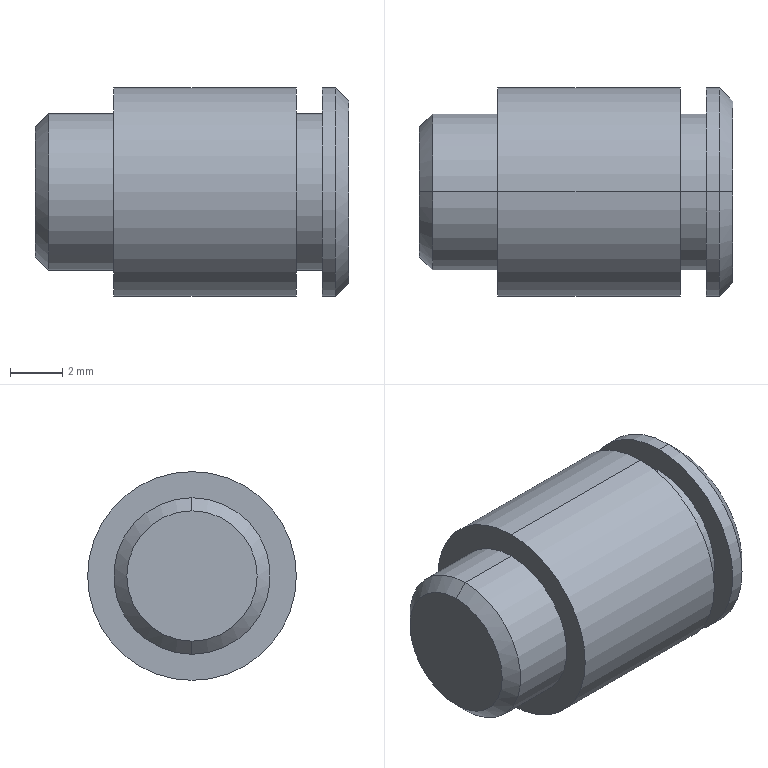Part | STEP file | 1 solid | 17 faces | box 12 x 8 x 8 mm | volume 509.985 mm3 | cylinder 8 | plane 5 | cone 4 | commonest cylinder face diameters 6 x4 8 x4
STEP:
#1=CARTESIAN_POINT('',(0.,0.,0.));
#2=DIRECTION('',(0.,0.,1.));
#3=DIRECTION('',(1.,0.,0.));
#4=AXIS2_PLACEMENT_3D('',#1,#2,#3);
#5=CARTESIAN_POINT('',(3.,0.,-4.));
#6=VERTEX_POINT('',#5);
#7=CARTESIAN_POINT('',(3.,0.,4.));
#8=VERTEX_POINT('',#7);
#9=CARTESIAN_POINT('',(3.,0.,0.));
#10=DIRECTION('',(1.,0.,0.));
#11=DIRECTION('',(0.,0.,-1.));
#12=AXIS2_PLACEMENT_3D('',#9,#10,#11);
#13=CIRCLE('',#12,4.);
#14=CARTESIAN_POINT('',(6.5,0.,0.));
#15=DIRECTION('',(1.,0.,0.));
#16=DIRECTION('',(0.,0.,-1.));
#17=AXIS2_PLACEMENT_3D('',#14,#15,#16);
#18=CYLINDRICAL_SURFACE('',#17,4.);
#19=CARTESIAN_POINT('',(0.,-3.5));
#20=DIRECTION('',(1.,0.));
#21=VECTOR('',#20,1.);
#22=LINE('',#19,#21);
#23=(GEOMETRIC_REPRESENTATION_CONTEXT(2)PARAMETRIC_REPRESENTATION_CONTEXT()REPRESENTATION_CONTEXT('',''));
#24=DEFINITIONAL_REPRESENTATION('',(#22),#23);
#25=PCURVE('',#18,#24);
#26=CARTESIAN_POINT('',(3.,3.5,0.));
#27=DIRECTION('',(-1.,0.,0.));
#28=DIRECTION('',(0.,0.,1.));
#29=AXIS2_PLACEMENT_3D('',#26,#27,#28);
#30=PLANE('',#29);
#31=CARTESIAN_POINT('',(-4.,-3.5));
#32=CARTESIAN_POINT('',(-4.,3.428));
#33=CARTESIAN_POINT('',(2.,-0.0359));
#34=CARTESIAN_POINT('',(8.,-3.5));
#35=CARTESIAN_POINT('',(2.,-6.964));
#36=CARTESIAN_POINT('',(-4.,-10.428));
#37=CARTESIAN_POINT('',(-4.,-3.5));
#38=(BOUNDED_CURVE()B_SPLINE_CURVE(2,(#31,#32,#33,#34,#35,#36,#37),.UNSPECIFIED.,.T.,.F.)B_SPLINE_CURVE_WITH_KNOTS((1,2,2,2,2,1),(-2.094,0.,2.094,4.189,6.283,8.378),.UNSPECIFIED.)CURVE()GEOMETRIC_REPRESENTATION_ITEM()RATIONAL_B_SPLINE_CURVE((1.,0.5,1.,0.5,1.,0.5,1.))REPRESENTATION_ITEM(''));
#39=(GEOMETRIC_REPRESENTATION_CONTEXT(2)PARAMETRIC_REPRESENTATION_CONTEXT()REPRESENTATION_CONTEXT('',''));
#40=DEFINITIONAL_REPRESENTATION('',(#38),#39);
#41=PCURVE('',#30,#40);
#42=SURFACE_CURVE('',#13,(#25,#41),.PCURVE_S1.);
#43=EDGE_CURVE('',#6,#8,#42,.T.);
#44=ORIENTED_EDGE('',*,*,#43,.T.);
#45=CARTESIAN_POINT('',(10.,0.,4.));
#46=VERTEX_POINT('',#45);
#47=CARTESIAN_POINT('',(6.5,0.,4.));
#48=DIRECTION('',(1.,0.,0.));
#49=VECTOR('',#48,1.);
#50=LINE('',#47,#49);
#51=CARTESIAN_POINT('',(3.142,0.));
#52=DIRECTION('',(0.,1.));
#53=VECTOR('',#52,1.);
#54=LINE('',#51,#53);
#55=(GEOMETRIC_REPRESENTATION_CONTEXT(2)PARAMETRIC_REPRESENTATION_CONTEXT()REPRESENTATION_CONTEXT('',''));
#56=DEFINITIONAL_REPRESENTATION('',(#54),#55);
#57=PCURVE('',#18,#56);
#58=CARTESIAN_POINT('',(6.5,0.,0.));
#59=DIRECTION('',(1.,0.,0.));
#60=DIRECTION('',(0.,0.,-1.));
#61=AXIS2_PLACEMENT_3D('',#58,#59,#60);
#62=CYLINDRICAL_SURFACE('',#61,4.);
#63=CARTESIAN_POINT('',(3.142,0.));
#64=DIRECTION('',(0.,1.));
#65=VECTOR('',#64,1.);
#66=LINE('',#63,#65);
#67=(GEOMETRIC_REPRESENTATION_CONTEXT(2)PARAMETRIC_REPRESENTATION_CONTEXT()REPRESENTATION_CONTEXT('',''));
#68=DEFINITIONAL_REPRESENTATION('',(#66),#67);
#69=PCURVE('',#62,#68);
#70=SURFACE_CURVE('',#50,(#57,#69),.PCURVE_S1.);
#71=EDGE_CURVE('',#8,#46,#70,.T.);
#72=ORIENTED_EDGE('',*,*,#71,.T.);
#73=CARTESIAN_POINT('',(10.,0.,-4.));
#74=VERTEX_POINT('',#73);
#75=CARTESIAN_POINT('',(10.,0.,0.));
#76=DIRECTION('',(-1.,0.,0.));
#77=DIRECTION('',(0.,0.,-1.));
#78=AXIS2_PLACEMENT_3D('',#75,#76,#77);
#79=CIRCLE('',#78,4.);
#80=CARTESIAN_POINT('',(6.283,3.5));
#81=DIRECTION('',(-1.,0.));
#82=VECTOR('',#81,1.);
#83=LINE('',#80,#82);
#84=(GEOMETRIC_REPRESENTATION_CONTEXT(2)PARAMETRIC_REPRESENTATION_CONTEXT()REPRESENTATION_CONTEXT('',''));
#85=DEFINITIONAL_REPRESENTATION('',(#83),#84);
#86=PCURVE('',#18,#85);
#87=CARTESIAN_POINT('',(10.,3.5,0.));
#88=DIRECTION('',(1.,0.,0.));
#89=DIRECTION('',(0.,0.,-1.));
#90=AXIS2_PLACEMENT_3D('',#87,#88,#89);
#91=PLANE('',#90);
#92=CARTESIAN_POINT('',(4.,-3.5));
#93=CARTESIAN_POINT('',(4.,-10.428));
#94=CARTESIAN_POINT('',(-2.,-6.964));
#95=CARTESIAN_POINT('',(-8.,-3.5));
#96=CARTESIAN_POINT('',(-2.,-0.0359));
#97=CARTESIAN_POINT('',(4.,3.428));
#98=CARTESIAN_POINT('',(4.,-3.5));
#99=(BOUNDED_CURVE()B_SPLINE_CURVE(2,(#92,#93,#94,#95,#96,#97,#98),.UNSPECIFIED.,.T.,.F.)B_SPLINE_CURVE_WITH_KNOTS((1,2,2,2,2,1),(-2.094,0.,2.094,4.189,6.283,8.378),.UNSPECIFIED.)CURVE()GEOMETRIC_REPRESENTATION_ITEM()RATIONAL_B_SPLINE_CURVE((1.,0.5,1.,0.5,1.,0.5,1.))REPRESENTATION_ITEM(''));
#100=(GEOMETRIC_REPRESENTATION_CONTEXT(2)PARAMETRIC_REPRESENTATION_CONTEXT()REPRESENTATION_CONTEXT('',''));
#101=DEFINITIONAL_REPRESENTATION('',(#99),#100);
#102=PCURVE('',#91,#101);
#103=SURFACE_CURVE('',#79,(#86,#102),.PCURVE_S1.);
#104=EDGE_CURVE('',#46,#74,#103,.T.);
#105=ORIENTED_EDGE('',*,*,#104,.T.);
#106=CARTESIAN_POINT('',(6.5,0.,-4.));
#107=DIRECTION('',(1.,0.,0.));
#108=VECTOR('',#107,1.);
#109=LINE('',#106,#108);
#110=CARTESIAN_POINT('',(0.,0.));
#111=DIRECTION('',(0.,1.));
#112=VECTOR('',#111,1.);
#113=LINE('',#110,#112);
#114=(GEOMETRIC_REPRESENTATION_CONTEXT(2)PARAMETRIC_REPRESENTATION_CONTEXT()REPRESENTATION_CONTEXT('',''));
#115=DEFINITIONAL_REPRESENTATION('',(#113),#114);
#116=PCURVE('',#18,#115);
#117=CARTESIAN_POINT('',(6.283,0.));
#118=DIRECTION('',(0.,1.));
#119=VECTOR('',#118,1.);
#120=LINE('',#117,#119);
#121=(GEOMETRIC_REPRESENTATION_CONTEXT(2)PARAMETRIC_REPRESENTATION_CONTEXT()REPRESENTATION_CONTEXT('',''));
#122=DEFINITIONAL_REPRESENTATION('',(#120),#121);
#123=PCURVE('',#62,#122);
#124=SURFACE_CURVE('',#109,(#116,#123),.PCURVE_S1.);
#125=EDGE_CURVE('',#6,#74,#124,.T.);
#126=ORIENTED_EDGE('',*,*,#125,.F.);
#127=EDGE_LOOP('',(#44,#72,#105,#126));
#128=FACE_BOUND('',#127,.T.);
#129=ADVANCED_FACE('',(#128),#18,.T.);
#130=CARTESIAN_POINT('',(0.5,0.,-3.));
#131=VERTEX_POINT('',#130);
#132=CARTESIAN_POINT('',(0.5,0.,3.));
#133=VERTEX_POINT('',#132);
#134=CARTESIAN_POINT('',(0.5,0.,0.));
#135=DIRECTION('',(1.,0.,0.));
#136=DIRECTION('',(0.,0.,-1.));
#137=AXIS2_PLACEMENT_3D('',#134,#135,#136);
#138=CIRCLE('',#137,3.);
#139=CARTESIAN_POINT('',(1.5,0.,0.));
#140=DIRECTION('',(1.,0.,0.));
#141=DIRECTION('',(0.,0.,-1.));
#142=AXIS2_PLACEMENT_3D('',#139,#140,#141);
#143=CYLINDRICAL_SURFACE('',#142,3.);
#144=CARTESIAN_POINT('',(0.,-1.));
#145=DIRECTION('',(1.,0.));
#146=VECTOR('',#145,1.);
#147=LINE('',#144,#146);
#148=(GEOMETRIC_REPRESENTATION_CONTEXT(2)PARAMETRIC_REPRESENTATION_CONTEXT()REPRESENTATION_CONTEXT('',''));
#149=DEFINITIONAL_REPRESENTATION('',(#147),#148);
#150=PCURVE('',#143,#149);
#151=CARTESIAN_POINT('',(0.5,0.,0.));
#152=DIRECTION('',(1.,0.,0.));
#153=DIRECTION('',(0.,0.,-1.));
#154=AXIS2_PLACEMENT_3D('',#151,#152,#153);
#155=CONICAL_SURFACE('',#154,3.,0.7854);
#156=CARTESIAN_POINT('',(0.,0.));
#157=DIRECTION('',(1.,0.));
#158=VECTOR('',#157,1.);
#159=LINE('',#156,#158);
#160=(GEOMETRIC_REPRESENTATION_CONTEXT(2)PARAMETRIC_REPRESENTATION_CONTEXT()REPRESENTATION_CONTEXT('',''));
#161=DEFINITIONAL_REPRESENTATION('',(#159),#160);
#162=PCURVE('',#155,#161);
#163=SURFACE_CURVE('',#138,(#150,#162),.PCURVE_S1.);
#164=EDGE_CURVE('',#131,#133,#163,.T.);
#165=ORIENTED_EDGE('',*,*,#164,.T.);
#166=CARTESIAN_POINT('',(3.,0.,3.));
#167=VERTEX_POINT('',#166);
#168=CARTESIAN_POINT('',(1.5,0.,3.));
#169=DIRECTION('',(1.,0.,0.));
#170=VECTOR('',#169,1.);
#171=LINE('',#168,#170);
#172=CARTESIAN_POINT('',(3.142,0.));
#173=DIRECTION('',(0.,1.));
#174=VECTOR('',#173,1.);
#175=LINE('',#172,#174);
#176=(GEOMETRIC_REPRESENTATION_CONTEXT(2)PARAMETRIC_REPRESENTATION_CONTEXT()REPRESENTATION_CONTEXT('',''));
#177=DEFINITIONAL_REPRESENTATION('',(#175),#176);
#178=PCURVE('',#143,#177);
#179=CARTESIAN_POINT('',(1.5,0.,0.));
#180=DIRECTION('',(1.,0.,0.));
#181=DIRECTION('',(0.,0.,-1.));
#182=AXIS2_PLACEMENT_3D('',#179,#180,#181);
#183=CYLINDRICAL_SURFACE('',#182,3.);
#184=CARTESIAN_POINT('',(3.142,0.));
#185=DIRECTION('',(0.,1.));
#186=VECTOR('',#185,1.);
#187=LINE('',#184,#186);
#188=(GEOMETRIC_REPRESENTATION_CONTEXT(2)PARAMETRIC_REPRESENTATION_CONTEXT()REPRESENTATION_CONTEXT('',''));
#189=DEFINITIONAL_REPRESENTATION('',(#187),#188);
#190=PCURVE('',#183,#189);
#191=SURFACE_CURVE('',#171,(#178,#190),.PCURVE_S1.);
#192=EDGE_CURVE('',#133,#167,#191,.T.);
#193=ORIENTED_EDGE('',*,*,#192,.T.);
#194=CARTESIAN_POINT('',(3.,0.,-3.));
#195=VERTEX_POINT('',#194);
#196=CARTESIAN_POINT('',(3.,0.,0.));
#197=DIRECTION('',(1.,0.,0.));
#198=DIRECTION('',(0.,0.,-1.));
#199=AXIS2_PLACEMENT_3D('',#196,#197,#198);
#200=CIRCLE('',#199,3.);
#201=CARTESIAN_POINT('',(0.,1.5));
#202=DIRECTION('',(1.,0.));
#203=VECTOR('',#202,1.);
#204=LINE('',#201,#203);
#205=(GEOMETRIC_REPRESENTATION_CONTEXT(2)PARAMETRIC_REPRESENTATION_CONTEXT()REPRESENTATION_CONTEXT('',''));
#206=DEFINITIONAL_REPRESENTATION('',(#204),#205);
#207=PCURVE('',#143,#206);
#208=CARTESIAN_POINT('',(-3.,-3.5));
#209=CARTESIAN_POINT('',(-3.,1.696));
#210=CARTESIAN_POINT('',(1.5,-0.9019));
#211=CARTESIAN_POINT('',(6.,-3.5));
#212=CARTESIAN_POINT('',(1.5,-6.098));
#213=CARTESIAN_POINT('',(-3.,-8.696));
#214=CARTESIAN_POINT('',(-3.,-3.5));
#215=(BOUNDED_CURVE()B_SPLINE_CURVE(2,(#208,#209,#210,#211,#212,#213,#214),.UNSPECIFIED.,.T.,.F.)B_SPLINE_CURVE_WITH_KNOTS((1,2,2,2,2,1),(-2.094,0.,2.094,4.189,6.283,8.378),.UNSPECIFIED.)CURVE()GEOMETRIC_REPRESENTATION_ITEM()RATIONAL_B_SPLINE_CURVE((1.,0.5,1.,0.5,1.,0.5,1.))REPRESENTATION_ITEM(''));
#216=(GEOMETRIC_REPRESENTATION_CONTEXT(2)PARAMETRIC_REPRESENTATION_CONTEXT()REPRESENTATION_CONTEXT('',''));
#217=DEFINITIONAL_REPRESENTATION('',(#215),#216);
#218=PCURVE('',#30,#217);
#219=SURFACE_CURVE('',#200,(#207,#218),.PCURVE_S1.);
#220=EDGE_CURVE('',#195,#167,#219,.T.);
#221=ORIENTED_EDGE('',*,*,#220,.F.);
#222=CARTESIAN_POINT('',(1.5,0.,-3.));
#223=DIRECTION('',(1.,0.,0.));
#224=VECTOR('',#223,1.);
#225=LINE('',#222,#224);
#226=CARTESIAN_POINT('',(0.,0.));
#227=DIRECTION('',(0.,1.));
#228=VECTOR('',#227,1.);
#229=LINE('',#226,#228);
#230=(GEOMETRIC_REPRESENTATION_CONTEXT(2)PARAMETRIC_REPRESENTATION_CONTEXT()REPRESENTATION_CONTEXT('',''));
#231=DEFINITIONAL_REPRESENTATION('',(#229),#230);
#232=PCURVE('',#143,#231);
#233=CARTESIAN_POINT('',(6.283,0.));
#234=DIRECTION('',(0.,1.));
#235=VECTOR('',#234,1.);
#236=LINE('',#233,#235);
#237=(GEOMETRIC_REPRESENTATION_CONTEXT(2)PARAMETRIC_REPRESENTATION_CONTEXT()REPRESENTATION_CONTEXT('',''));
#238=DEFINITIONAL_REPRESENTATION('',(#236),#237);
#239=PCURVE('',#183,#238);
#240=SURFACE_CURVE('',#225,(#232,#239),.PCURVE_S1.);
#241=EDGE_CURVE('',#131,#195,#240,.T.);
#242=ORIENTED_EDGE('',*,*,#241,.F.);
#243=EDGE_LOOP('',(#165,#193,#221,#242));
#244=FACE_BOUND('',#243,.T.);
#245=ADVANCED_FACE('',(#244),#143,.T.);
#246=CARTESIAN_POINT('',(10.,0.,3.));
#247=VERTEX_POINT('',#246);
#248=CARTESIAN_POINT('',(10.,0.,-3.));
#249=VERTEX_POINT('',#248);
#250=CARTESIAN_POINT('',(10.,0.,0.));
#251=DIRECTION('',(-1.,0.,0.));
#252=DIRECTION('',(0.,0.,-1.));
#253=AXIS2_PLACEMENT_3D('',#250,#251,#252);
#254=CIRCLE('',#253,3.);
#255=CARTESIAN_POINT('',(10.5,0.,0.));
#256=DIRECTION('',(1.,0.,0.));
#257=DIRECTION('',(0.,0.,-1.));
#258=AXIS2_PLACEMENT_3D('',#255,#256,#257);
#259=CYLINDRICAL_SURFACE('',#258,3.);
#260=CARTESIAN_POINT('',(6.283,-0.5));
#261=DIRECTION('',(-1.,0.));
#262=VECTOR('',#261,1.);
#263=LINE('',#260,#262);
#264=(GEOMETRIC_REPRESENTATION_CONTEXT(2)PARAMETRIC_REPRESENTATION_CONTEXT()REPRESENTATION_CONTEXT('',''));
#265=DEFINITIONAL_REPRESENTATION('',(#263),#264);
#266=PCURVE('',#259,#265);
#267=CARTESIAN_POINT('',(3.,-3.5));
#268=CARTESIAN_POINT('',(3.,-8.696));
#269=CARTESIAN_POINT('',(-1.5,-6.098));
#270=CARTESIAN_POINT('',(-6.,-3.5));
#271=CARTESIAN_POINT('',(-1.5,-0.9019));
#272=CARTESIAN_POINT('',(3.,1.696));
#273=CARTESIAN_POINT('',(3.,-3.5));
#274=(BOUNDED_CURVE()B_SPLINE_CURVE(2,(#267,#268,#269,#270,#271,#272,#273),.UNSPECIFIED.,.T.,.F.)B_SPLINE_CURVE_WITH_KNOTS((1,2,2,2,2,1),(-2.094,0.,2.094,4.189,6.283,8.378),.UNSPECIFIED.)CURVE()GEOMETRIC_REPRESENTATION_ITEM()RATIONAL_B_SPLINE_CURVE((1.,0.5,1.,0.5,1.,0.5,1.))REPRESENTATION_ITEM(''));
#275=(GEOMETRIC_REPRESENTATION_CONTEXT(2)PARAMETRIC_REPRESENTATION_CONTEXT()REPRESENTATION_CONTEXT('',''));
#276=DEFINITIONAL_REPRESENTATION('',(#274),#275);
#277=PCURVE('',#91,#276);
#278=SURFACE_CURVE('',#254,(#266,#277),.PCURVE_S1.);
#279=EDGE_CURVE('',#247,#249,#278,.T.);
#280=ORIENTED_EDGE('',*,*,#279,.F.);
#281=CARTESIAN_POINT('',(11.,0.,3.));
#282=VERTEX_POINT('',#281);
#283=CARTESIAN_POINT('',(10.5,0.,3.));
#284=DIRECTION('',(1.,0.,0.));
#285=VECTOR('',#284,1.);
#286=LINE('',#283,#285);
#287=CARTESIAN_POINT('',(3.142,0.));
#288=DIRECTION('',(0.,1.));
#289=VECTOR('',#288,1.);
#290=LINE('',#287,#289);
#291=(GEOMETRIC_REPRESENTATION_CONTEXT(2)PARAMETRIC_REPRESENTATION_CONTEXT()REPRESENTATION_CONTEXT('',''));
#292=DEFINITIONAL_REPRESENTATION('',(#290),#291);
#293=PCURVE('',#259,#292);
#294=CARTESIAN_POINT('',(10.5,0.,0.));
#295=DIRECTION('',(1.,0.,0.));
#296=DIRECTION('',(0.,0.,-1.));
#297=AXIS2_PLACEMENT_3D('',#294,#295,#296);
#298=CYLINDRICAL_SURFACE('',#297,3.);
#299=CARTESIAN_POINT('',(3.142,0.));
#300=DIRECTION('',(0.,1.));
#301=VECTOR('',#300,1.);
#302=LINE('',#299,#301);
#303=(GEOMETRIC_REPRESENTATION_CONTEXT(2)PARAMETRIC_REPRESENTATION_CONTEXT()REPRESENTATION_CONTEXT('',''));
#304=DEFINITIONAL_REPRESENTATION('',(#302),#303);
#305=PCURVE('',#298,#304);
#306=SURFACE_CURVE('',#286,(#293,#305),.PCURVE_S1.);
#307=EDGE_CURVE('',#247,#282,#306,.T.);
#308=ORIENTED_EDGE('',*,*,#307,.T.);
#309=CARTESIAN_POINT('',(11.,0.,-3.));
#310=VERTEX_POINT('',#309);
#311=CARTESIAN_POINT('',(11.,0.,0.));
#312=DIRECTION('',(-1.,0.,0.));
#313=DIRECTION('',(0.,0.,-1.));
#314=AXIS2_PLACEMENT_3D('',#311,#312,#313);
#315=CIRCLE('',#314,3.);
#316=CARTESIAN_POINT('',(6.283,0.5));
#317=DIRECTION('',(-1.,0.));
#318=VECTOR('',#317,1.);
#319=LINE('',#316,#318);
#320=(GEOMETRIC_REPRESENTATION_CONTEXT(2)PARAMETRIC_REPRESENTATION_CONTEXT()REPRESENTATION_CONTEXT('',''));
#321=DEFINITIONAL_REPRESENTATION('',(#319),#320);
#322=PCURVE('',#259,#321);
#323=CARTESIAN_POINT('',(11.,3.5,0.));
#324=DIRECTION('',(-1.,0.,0.));
#325=DIRECTION('',(0.,0.,1.));
#326=AXIS2_PLACEMENT_3D('',#323,#324,#325);
#327=PLANE('',#326);
#328=CARTESIAN_POINT('',(0.,-3.5));
#329=DIRECTION('',(-1.,0.));
#330=AXIS2_PLACEMENT_2D('',#328,#329);
#331=CIRCLE('',#330,3.);
#332=(GEOMETRIC_REPRESENTATION_CONTEXT(2)PARAMETRIC_REPRESENTATION_CONTEXT()REPRESENTATION_CONTEXT('',''));
#333=DEFINITIONAL_REPRESENTATION('',(#331),#332);
#334=PCURVE('',#327,#333);
#335=SURFACE_CURVE('',#315,(#322,#334),.PCURVE_S1.);
#336=EDGE_CURVE('',#282,#310,#335,.T.);
#337=ORIENTED_EDGE('',*,*,#336,.T.);
#338=CARTESIAN_POINT('',(10.5,0.,-3.));
#339=DIRECTION('',(1.,0.,0.));
#340=VECTOR('',#339,1.);
#341=LINE('',#338,#340);
#342=CARTESIAN_POINT('',(0.,0.));
#343=DIRECTION('',(0.,1.));
#344=VECTOR('',#343,1.);
#345=LINE('',#342,#344);
#346=(GEOMETRIC_REPRESENTATION_CONTEXT(2)PARAMETRIC_REPRESENTATION_CONTEXT()REPRESENTATION_CONTEXT('',''));
#347=DEFINITIONAL_REPRESENTATION('',(#345),#346);
#348=PCURVE('',#259,#347);
#349=CARTESIAN_POINT('',(6.283,0.));
#350=DIRECTION('',(0.,1.));
#351=VECTOR('',#350,1.);
#352=LINE('',#349,#351);
#353=(GEOMETRIC_REPRESENTATION_CONTEXT(2)PARAMETRIC_REPRESENTATION_CONTEXT()REPRESENTATION_CONTEXT('',''));
#354=DEFINITIONAL_REPRESENTATION('',(#352),#353);
#355=PCURVE('',#298,#354);
#356=SURFACE_CURVE('',#341,(#348,#355),.PCURVE_S1.);
#357=EDGE_CURVE('',#249,#310,#356,.T.);
#358=ORIENTED_EDGE('',*,*,#357,.F.);
#359=EDGE_LOOP('',(#280,#308,#337,#358));
#360=FACE_BOUND('',#359,.T.);
#361=ADVANCED_FACE('',(#360),#259,.T.);
#362=CARTESIAN_POINT('',(0.,0.,-2.5));
#363=VERTEX_POINT('',#362);
#364=CARTESIAN_POINT('',(0.,0.,2.5));
#365=VERTEX_POINT('',#364);
#366=CARTESIAN_POINT('',(0.,0.,0.));
#367=DIRECTION('',(1.,0.,0.));
#368=DIRECTION('',(0.,0.,-1.));
#369=AXIS2_PLACEMENT_3D('',#366,#367,#368);
#370=CIRCLE('',#369,2.5);
#371=CARTESIAN_POINT('',(0.,-0.5));
#372=DIRECTION('',(1.,0.));
#373=VECTOR('',#372,1.);
#374=LINE('',#371,#373);
#375=(GEOMETRIC_REPRESENTATION_CONTEXT(2)PARAMETRIC_REPRESENTATION_CONTEXT()REPRESENTATION_CONTEXT('',''));
#376=DEFINITIONAL_REPRESENTATION('',(#374),#375);
#377=PCURVE('',#155,#376);
#378=CARTESIAN_POINT('',(0.,1.5,0.));
#379=DIRECTION('',(-1.,0.,0.));
#380=DIRECTION('',(0.,0.,1.));
#381=AXIS2_PLACEMENT_3D('',#378,#379,#380);
#382=PLANE('',#381);
#383=CARTESIAN_POINT('',(-2.5,-1.5));
#384=CARTESIAN_POINT('',(-2.5,2.83));
#385=CARTESIAN_POINT('',(1.25,0.6651));
#386=CARTESIAN_POINT('',(5.,-1.5));
#387=CARTESIAN_POINT('',(1.25,-3.665));
#388=CARTESIAN_POINT('',(-2.5,-5.83));
#389=CARTESIAN_POINT('',(-2.5,-1.5));
#390=(BOUNDED_CURVE()B_SPLINE_CURVE(2,(#383,#384,#385,#386,#387,#388,#389),.UNSPECIFIED.,.T.,.F.)B_SPLINE_CURVE_WITH_KNOTS((1,2,2,2,2,1),(-2.094,0.,2.094,4.189,6.283,8.378),.UNSPECIFIED.)CURVE()GEOMETRIC_REPRESENTATION_ITEM()RATIONAL_B_SPLINE_CURVE((1.,0.5,1.,0.5,1.,0.5,1.))REPRESENTATION_ITEM(''));
#391=(GEOMETRIC_REPRESENTATION_CONTEXT(2)PARAMETRIC_REPRESENTATION_CONTEXT()REPRESENTATION_CONTEXT('',''));
#392=DEFINITIONAL_REPRESENTATION('',(#390),#391);
#393=PCURVE('',#382,#392);
#394=SURFACE_CURVE('',#370,(#377,#393),.PCURVE_S1.);
#395=EDGE_CURVE('',#363,#365,#394,.T.);
#396=ORIENTED_EDGE('',*,*,#395,.T.);
#397=CARTESIAN_POINT('',(0.5,0.,3.));
#398=DIRECTION('',(0.7071,0.,0.7071));
#399=VECTOR('',#398,1.);
#400=LINE('',#397,#399);
#401=CARTESIAN_POINT('',(3.142,0.));
#402=DIRECTION('',(0.,1.));
#403=VECTOR('',#402,1.);
#404=LINE('',#401,#403);
#405=(GEOMETRIC_REPRESENTATION_CONTEXT(2)PARAMETRIC_REPRESENTATION_CONTEXT()REPRESENTATION_CONTEXT('',''));
#406=DEFINITIONAL_REPRESENTATION('',(#404),#405);
#407=PCURVE('',#155,#406);
#408=CARTESIAN_POINT('',(0.5,0.,0.));
#409=DIRECTION('',(1.,0.,0.));
#410=DIRECTION('',(0.,0.,-1.));
#411=AXIS2_PLACEMENT_3D('',#408,#409,#410);
#412=CONICAL_SURFACE('',#411,3.,0.7854);
#413=CARTESIAN_POINT('',(3.142,0.));
#414=DIRECTION('',(0.,1.));
#415=VECTOR('',#414,1.);
#416=LINE('',#413,#415);
#417=(GEOMETRIC_REPRESENTATION_CONTEXT(2)PARAMETRIC_REPRESENTATION_CONTEXT()REPRESENTATION_CONTEXT('',''));
#418=DEFINITIONAL_REPRESENTATION('',(#416),#417);
#419=PCURVE('',#412,#418);
#420=SURFACE_CURVE('',#400,(#407,#419),.PCURVE_S1.);
#421=EDGE_CURVE('',#365,#133,#420,.T.);
#422=ORIENTED_EDGE('',*,*,#421,.T.);
#423=ORIENTED_EDGE('',*,*,#164,.F.);
#424=CARTESIAN_POINT('',(0.5,0.,-3.));
#425=DIRECTION('',(0.7071,0.,-0.7071));
#426=VECTOR('',#425,1.);
#427=LINE('',#424,#426);
#428=CARTESIAN_POINT('',(0.,0.));
#429=DIRECTION('',(0.,1.));
#430=VECTOR('',#429,1.);
#431=LINE('',#428,#430);
#432=(GEOMETRIC_REPRESENTATION_CONTEXT(2)PARAMETRIC_REPRESENTATION_CONTEXT()REPRESENTATION_CONTEXT('',''));
#433=DEFINITIONAL_REPRESENTATION('',(#431),#432);
#434=PCURVE('',#155,#433);
#435=CARTESIAN_POINT('',(6.283,0.));
#436=DIRECTION('',(0.,1.));
#437=VECTOR('',#436,1.);
#438=LINE('',#435,#437);
#439=(GEOMETRIC_REPRESENTATION_CONTEXT(2)PARAMETRIC_REPRESENTATION_CONTEXT()REPRESENTATION_CONTEXT('',''));
#440=DEFINITIONAL_REPRESENTATION('',(#438),#439);
#441=PCURVE('',#412,#440);
#442=SURFACE_CURVE('',#427,(#434,#441),.PCURVE_S1.);
#443=EDGE_CURVE('',#363,#131,#442,.T.);
#444=ORIENTED_EDGE('',*,*,#443,.F.);
#445=EDGE_LOOP('',(#396,#422,#423,#444));
#446=FACE_BOUND('',#445,.T.);
#447=ADVANCED_FACE('',(#446),#155,.T.);
#448=CARTESIAN_POINT('',(11.,0.,4.));
#449=VERTEX_POINT('',#448);
#450=CARTESIAN_POINT('',(11.,0.,-4.));
#451=VERTEX_POINT('',#450);
#452=CARTESIAN_POINT('',(11.,0.,0.));
#453=DIRECTION('',(-1.,0.,0.));
#454=DIRECTION('',(0.,0.,-1.));
#455=AXIS2_PLACEMENT_3D('',#452,#453,#454);
#456=CIRCLE('',#455,4.);
#457=CARTESIAN_POINT('',(11.5,0.,0.));
#458=DIRECTION('',(1.,0.,0.));
#459=DIRECTION('',(0.,0.,-1.));
#460=AXIS2_PLACEMENT_3D('',#457,#458,#459);
#461=CYLINDRICAL_SURFACE('',#460,4.);
#462=CARTESIAN_POINT('',(6.283,-0.5));
#463=DIRECTION('',(-1.,0.));
#464=VECTOR('',#463,1.);
#465=LINE('',#462,#464);
#466=(GEOMETRIC_REPRESENTATION_CONTEXT(2)PARAMETRIC_REPRESENTATION_CONTEXT()REPRESENTATION_CONTEXT('',''));
#467=DEFINITIONAL_REPRESENTATION('',(#465),#466);
#468=PCURVE('',#461,#467);
#469=CARTESIAN_POINT('',(0.,-3.5));
#470=DIRECTION('',(-1.,0.));
#471=AXIS2_PLACEMENT_2D('',#469,#470);
#472=CIRCLE('',#471,4.);
#473=(GEOMETRIC_REPRESENTATION_CONTEXT(2)PARAMETRIC_REPRESENTATION_CONTEXT()REPRESENTATION_CONTEXT('',''));
#474=DEFINITIONAL_REPRESENTATION('',(#472),#473);
#475=PCURVE('',#327,#474);
#476=SURFACE_CURVE('',#456,(#468,#475),.PCURVE_S1.);
#477=EDGE_CURVE('',#449,#451,#476,.T.);
#478=ORIENTED_EDGE('',*,*,#477,.F.);
#479=CARTESIAN_POINT('',(11.5,0.,4.));
#480=VERTEX_POINT('',#479);
#481=CARTESIAN_POINT('',(11.5,0.,4.));
#482=DIRECTION('',(1.,0.,0.));
#483=VECTOR('',#482,1.);
#484=LINE('',#481,#483);
#485=CARTESIAN_POINT('',(3.142,0.));
#486=DIRECTION('',(0.,1.));
#487=VECTOR('',#486,1.);
#488=LINE('',#485,#487);
#489=(GEOMETRIC_REPRESENTATION_CONTEXT(2)PARAMETRIC_REPRESENTATION_CONTEXT()REPRESENTATION_CONTEXT('',''));
#490=DEFINITIONAL_REPRESENTATION('',(#488),#489);
#491=PCURVE('',#461,#490);
#492=CARTESIAN_POINT('',(11.5,0.,0.));
#493=DIRECTION('',(1.,0.,0.));
#494=DIRECTION('',(0.,0.,-1.));
#495=AXIS2_PLACEMENT_3D('',#492,#493,#494);
#496=CYLINDRICAL_SURFACE('',#495,4.);
#497=CARTESIAN_POINT('',(3.142,0.));
#498=DIRECTION('',(0.,1.));
#499=VECTOR('',#498,1.);
#500=LINE('',#497,#499);
#501=(GEOMETRIC_REPRESENTATION_CONTEXT(2)PARAMETRIC_REPRESENTATION_CONTEXT()REPRESENTATION_CONTEXT('',''));
#502=DEFINITIONAL_REPRESENTATION('',(#500),#501);
#503=PCURVE('',#496,#502);
#504=SURFACE_CURVE('',#484,(#491,#503),.PCURVE_S1.);
#505=EDGE_CURVE('',#449,#480,#504,.T.);
#506=ORIENTED_EDGE('',*,*,#505,.T.);
#507=CARTESIAN_POINT('',(11.5,0.,-4.));
#508=VERTEX_POINT('',#507);
#509=CARTESIAN_POINT('',(11.5,0.,0.));
#510=DIRECTION('',(-1.,0.,0.));
#511=DIRECTION('',(0.,0.,-1.));
#512=AXIS2_PLACEMENT_3D('',#509,#510,#511);
#513=CIRCLE('',#512,4.);
#514=CARTESIAN_POINT('',(6.283,0.));
#515=DIRECTION('',(-1.,0.));
#516=VECTOR('',#515,1.);
#517=LINE('',#514,#516);
#518=(GEOMETRIC_REPRESENTATION_CONTEXT(2)PARAMETRIC_REPRESENTATION_CONTEXT()REPRESENTATION_CONTEXT('',''));
#519=DEFINITIONAL_REPRESENTATION('',(#517),#518);
#520=PCURVE('',#461,#519);
#521=CARTESIAN_POINT('',(11.5,0.,0.));
#522=DIRECTION('',(-1.,0.,0.));
#523=DIRECTION('',(0.,0.,1.));
#524=AXIS2_PLACEMENT_3D('',#521,#522,#523);
#525=CONICAL_SURFACE('',#524,4.,0.7854);
#526=CARTESIAN_POINT('',(-3.142,0.));
#527=DIRECTION('',(1.,0.));
#528=VECTOR('',#527,1.);
#529=LINE('',#526,#528);
#530=(GEOMETRIC_REPRESENTATION_CONTEXT(2)PARAMETRIC_REPRESENTATION_CONTEXT()REPRESENTATION_CONTEXT('',''));
#531=DEFINITIONAL_REPRESENTATION('',(#529),#530);
#532=PCURVE('',#525,#531);
#533=SURFACE_CURVE('',#513,(#520,#532),.PCURVE_S1.);
#534=EDGE_CURVE('',#480,#508,#533,.T.);
#535=ORIENTED_EDGE('',*,*,#534,.T.);
#536=CARTESIAN_POINT('',(11.5,0.,-4.));
#537=DIRECTION('',(1.,0.,0.));
#538=VECTOR('',#537,1.);
#539=LINE('',#536,#538);
#540=CARTESIAN_POINT('',(0.,0.));
#541=DIRECTION('',(0.,1.));
#542=VECTOR('',#541,1.);
#543=LINE('',#540,#542);
#544=(GEOMETRIC_REPRESENTATION_CONTEXT(2)PARAMETRIC_REPRESENTATION_CONTEXT()REPRESENTATION_CONTEXT('',''));
#545=DEFINITIONAL_REPRESENTATION('',(#543),#544);
#546=PCURVE('',#461,#545);
#547=CARTESIAN_POINT('',(6.283,0.));
#548=DIRECTION('',(0.,1.));
#549=VECTOR('',#548,1.);
#550=LINE('',#547,#549);
#551=(GEOMETRIC_REPRESENTATION_CONTEXT(2)PARAMETRIC_REPRESENTATION_CONTEXT()REPRESENTATION_CONTEXT('',''));
#552=DEFINITIONAL_REPRESENTATION('',(#550),#551);
#553=PCURVE('',#496,#552);
#554=SURFACE_CURVE('',#539,(#546,#553),.PCURVE_S1.);
#555=EDGE_CURVE('',#451,#508,#554,.T.);
#556=ORIENTED_EDGE('',*,*,#555,.F.);
#557=EDGE_LOOP('',(#478,#506,#535,#556));
#558=FACE_BOUND('',#557,.T.);
#559=ADVANCED_FACE('',(#558),#461,.T.);
#560=CARTESIAN_POINT('',(12.,0.,3.5));
#561=VERTEX_POINT('',#560);
#562=CARTESIAN_POINT('',(12.,0.,-3.5));
#563=VERTEX_POINT('',#562);
#564=CARTESIAN_POINT('',(12.,0.,0.));
#565=DIRECTION('',(-1.,0.,0.));
#566=DIRECTION('',(0.,0.,1.));
#567=AXIS2_PLACEMENT_3D('',#564,#565,#566);
#568=CIRCLE('',#567,3.5);
#569=CARTESIAN_POINT('',(0.,-0.5));
#570=DIRECTION('',(1.,0.));
#571=VECTOR('',#570,1.);
#572=LINE('',#569,#571);
#573=(GEOMETRIC_REPRESENTATION_CONTEXT(2)PARAMETRIC_REPRESENTATION_CONTEXT()REPRESENTATION_CONTEXT('',''));
#574=DEFINITIONAL_REPRESENTATION('',(#572),#573);
#575=PCURVE('',#525,#574);
#576=CARTESIAN_POINT('',(12.,2.,0.));
#577=DIRECTION('',(1.,0.,0.));
#578=DIRECTION('',(0.,0.,-1.));
#579=AXIS2_PLACEMENT_3D('',#576,#577,#578);
#580=PLANE('',#579);
#581=CARTESIAN_POINT('',(-3.5,-2.));
#582=CARTESIAN_POINT('',(-3.5,4.062));
#583=CARTESIAN_POINT('',(1.75,1.031));
#584=CARTESIAN_POINT('',(7.,-2.));
#585=CARTESIAN_POINT('',(1.75,-5.031));
#586=CARTESIAN_POINT('',(-3.5,-8.062));
#587=CARTESIAN_POINT('',(-3.5,-2.));
#588=(BOUNDED_CURVE()B_SPLINE_CURVE(2,(#581,#582,#583,#584,#585,#586,#587),.UNSPECIFIED.,.T.,.F.)B_SPLINE_CURVE_WITH_KNOTS((1,2,2,2,2,1),(-2.094,0.,2.094,4.189,6.283,8.378),.UNSPECIFIED.)CURVE()GEOMETRIC_REPRESENTATION_ITEM()RATIONAL_B_SPLINE_CURVE((1.,0.5,1.,0.5,1.,0.5,1.))REPRESENTATION_ITEM(''));
#589=(GEOMETRIC_REPRESENTATION_CONTEXT(2)PARAMETRIC_REPRESENTATION_CONTEXT()REPRESENTATION_CONTEXT('',''));
#590=DEFINITIONAL_REPRESENTATION('',(#588),#589);
#591=PCURVE('',#580,#590);
#592=SURFACE_CURVE('',#568,(#575,#591),.PCURVE_S1.);
#593=EDGE_CURVE('',#561,#563,#592,.T.);
#594=ORIENTED_EDGE('',*,*,#593,.T.);
#595=CARTESIAN_POINT('',(11.5,0.,-4.));
#596=DIRECTION('',(-0.7071,0.,-0.7071));
#597=VECTOR('',#596,1.);
#598=LINE('',#595,#597);
#599=CARTESIAN_POINT('',(3.142,0.));
#600=DIRECTION('',(0.,1.));
#601=VECTOR('',#600,1.);
#602=LINE('',#599,#601);
#603=(GEOMETRIC_REPRESENTATION_CONTEXT(2)PARAMETRIC_REPRESENTATION_CONTEXT()REPRESENTATION_CONTEXT('',''));
#604=DEFINITIONAL_REPRESENTATION('',(#602),#603);
#605=PCURVE('',#525,#604);
#606=CARTESIAN_POINT('',(11.5,0.,0.));
#607=DIRECTION('',(-1.,0.,0.));
#608=DIRECTION('',(0.,0.,1.));
#609=AXIS2_PLACEMENT_3D('',#606,#607,#608);
#610=CONICAL_SURFACE('',#609,4.,0.7854);
#611=CARTESIAN_POINT('',(3.142,0.));
#612=DIRECTION('',(0.,1.));
#613=VECTOR('',#612,1.);
#614=LINE('',#611,#613);
#615=(GEOMETRIC_REPRESENTATION_CONTEXT(2)PARAMETRIC_REPRESENTATION_CONTEXT()REPRESENTATION_CONTEXT('',''));
#616=DEFINITIONAL_REPRESENTATION('',(#614),#615);
#617=PCURVE('',#610,#616);
#618=SURFACE_CURVE('',#598,(#605,#617),.PCURVE_S1.);
#619=EDGE_CURVE('',#563,#508,#618,.T.);
#620=ORIENTED_EDGE('',*,*,#619,.T.);
#621=ORIENTED_EDGE('',*,*,#534,.F.);
#622=CARTESIAN_POINT('',(11.5,0.,4.));
#623=DIRECTION('',(-0.7071,0.,0.7071));
#624=VECTOR('',#623,1.);
#625=LINE('',#622,#624);
#626=CARTESIAN_POINT('',(0.,0.));
#627=DIRECTION('',(0.,1.));
#628=VECTOR('',#627,1.);
#629=LINE('',#626,#628);
#630=(GEOMETRIC_REPRESENTATION_CONTEXT(2)PARAMETRIC_REPRESENTATION_CONTEXT()REPRESENTATION_CONTEXT('',''));
#631=DEFINITIONAL_REPRESENTATION('',(#629),#630);
#632=PCURVE('',#525,#631);
#633=CARTESIAN_POINT('',(6.283,0.));
#634=DIRECTION('',(0.,1.));
#635=VECTOR('',#634,1.);
#636=LINE('',#633,#635);
#637=(GEOMETRIC_REPRESENTATION_CONTEXT(2)PARAMETRIC_REPRESENTATION_CONTEXT()REPRESENTATION_CONTEXT('',''));
#638=DEFINITIONAL_REPRESENTATION('',(#636),#637);
#639=PCURVE('',#610,#638);
#640=SURFACE_CURVE('',#625,(#632,#639),.PCURVE_S1.);
#641=EDGE_CURVE('',#561,#480,#640,.T.);
#642=ORIENTED_EDGE('',*,*,#641,.F.);
#643=EDGE_LOOP('',(#594,#620,#621,#642));
#644=FACE_BOUND('',#643,.T.);
#645=ADVANCED_FACE('',(#644),#525,.T.);
#646=ORIENTED_EDGE('',*,*,#71,.F.);
#647=CARTESIAN_POINT('',(3.,0.,0.));
#648=DIRECTION('',(1.,0.,0.));
#649=DIRECTION('',(0.,0.,-1.));
#650=AXIS2_PLACEMENT_3D('',#647,#648,#649);
#651=CIRCLE('',#650,4.);
#652=CARTESIAN_POINT('',(0.,-3.5));
#653=DIRECTION('',(1.,0.));
#654=VECTOR('',#653,1.);
#655=LINE('',#652,#654);
#656=(GEOMETRIC_REPRESENTATION_CONTEXT(2)PARAMETRIC_REPRESENTATION_CONTEXT()REPRESENTATION_CONTEXT('',''));
#657=DEFINITIONAL_REPRESENTATION('',(#655),#656);
#658=PCURVE('',#62,#657);
#659=CARTESIAN_POINT('',(-4.,-3.5));
#660=CARTESIAN_POINT('',(-4.,3.428));
#661=CARTESIAN_POINT('',(2.,-0.0359));
#662=CARTESIAN_POINT('',(8.,-3.5));
#663=CARTESIAN_POINT('',(2.,-6.964));
#664=CARTESIAN_POINT('',(-4.,-10.428));
#665=CARTESIAN_POINT('',(-4.,-3.5));
#666=(BOUNDED_CURVE()B_SPLINE_CURVE(2,(#659,#660,#661,#662,#663,#664,#665),.UNSPECIFIED.,.T.,.F.)B_SPLINE_CURVE_WITH_KNOTS((1,2,2,2,2,1),(-2.094,0.,2.094,4.189,6.283,8.378),.UNSPECIFIED.)CURVE()GEOMETRIC_REPRESENTATION_ITEM()RATIONAL_B_SPLINE_CURVE((1.,0.5,1.,0.5,1.,0.5,1.))REPRESENTATION_ITEM(''));
#667=(GEOMETRIC_REPRESENTATION_CONTEXT(2)PARAMETRIC_REPRESENTATION_CONTEXT()REPRESENTATION_CONTEXT('',''));
#668=DEFINITIONAL_REPRESENTATION('',(#666),#667);
#669=PCURVE('',#30,#668);
#670=SURFACE_CURVE('',#651,(#658,#669),.PCURVE_S1.);
#671=EDGE_CURVE('',#8,#6,#670,.T.);
#672=ORIENTED_EDGE('',*,*,#671,.T.);
#673=ORIENTED_EDGE('',*,*,#125,.T.);
#674=CARTESIAN_POINT('',(10.,0.,0.));
#675=DIRECTION('',(-1.,0.,0.));
#676=DIRECTION('',(0.,0.,-1.));
#677=AXIS2_PLACEMENT_3D('',#674,#675,#676);
#678=CIRCLE('',#677,4.);
#679=CARTESIAN_POINT('',(6.283,3.5));
#680=DIRECTION('',(-1.,0.));
#681=VECTOR('',#680,1.);
#682=LINE('',#679,#681);
#683=(GEOMETRIC_REPRESENTATION_CONTEXT(2)PARAMETRIC_REPRESENTATION_CONTEXT()REPRESENTATION_CONTEXT('',''));
#684=DEFINITIONAL_REPRESENTATION('',(#682),#683);
#685=PCURVE('',#62,#684);
#686=CARTESIAN_POINT('',(4.,-3.5));
#687=CARTESIAN_POINT('',(4.,-10.428));
#688=CARTESIAN_POINT('',(-2.,-6.964));
#689=CARTESIAN_POINT('',(-8.,-3.5));
#690=CARTESIAN_POINT('',(-2.,-0.0359));
#691=CARTESIAN_POINT('',(4.,3.428));
#692=CARTESIAN_POINT('',(4.,-3.5));
#693=(BOUNDED_CURVE()B_SPLINE_CURVE(2,(#686,#687,#688,#689,#690,#691,#692),.UNSPECIFIED.,.T.,.F.)B_SPLINE_CURVE_WITH_KNOTS((1,2,2,2,2,1),(-2.094,0.,2.094,4.189,6.283,8.378),.UNSPECIFIED.)CURVE()GEOMETRIC_REPRESENTATION_ITEM()RATIONAL_B_SPLINE_CURVE((1.,0.5,1.,0.5,1.,0.5,1.))REPRESENTATION_ITEM(''));
#694=(GEOMETRIC_REPRESENTATION_CONTEXT(2)PARAMETRIC_REPRESENTATION_CONTEXT()REPRESENTATION_CONTEXT('',''));
#695=DEFINITIONAL_REPRESENTATION('',(#693),#694);
#696=PCURVE('',#91,#695);
#697=SURFACE_CURVE('',#678,(#685,#696),.PCURVE_S1.);
#698=EDGE_CURVE('',#74,#46,#697,.T.);
#699=ORIENTED_EDGE('',*,*,#698,.T.);
#700=EDGE_LOOP('',(#646,#672,#673,#699));
#701=FACE_BOUND('',#700,.T.);
#702=ADVANCED_FACE('',(#701),#62,.T.);
#703=ORIENTED_EDGE('',*,*,#220,.T.);
#704=CARTESIAN_POINT('',(3.,0.,0.));
#705=DIRECTION('',(1.,0.,0.));
#706=DIRECTION('',(0.,0.,-1.));
#707=AXIS2_PLACEMENT_3D('',#704,#705,#706);
#708=CIRCLE('',#707,3.);
#709=CARTESIAN_POINT('',(-3.,-3.5));
#710=CARTESIAN_POINT('',(-3.,1.696));
#711=CARTESIAN_POINT('',(1.5,-0.9019));
#712=CARTESIAN_POINT('',(6.,-3.5));
#713=CARTESIAN_POINT('',(1.5,-6.098));
#714=CARTESIAN_POINT('',(-3.,-8.696));
#715=CARTESIAN_POINT('',(-3.,-3.5));
#716=(BOUNDED_CURVE()B_SPLINE_CURVE(2,(#709,#710,#711,#712,#713,#714,#715),.UNSPECIFIED.,.T.,.F.)B_SPLINE_CURVE_WITH_KNOTS((1,2,2,2,2,1),(-2.094,0.,2.094,4.189,6.283,8.378),.UNSPECIFIED.)CURVE()GEOMETRIC_REPRESENTATION_ITEM()RATIONAL_B_SPLINE_CURVE((1.,0.5,1.,0.5,1.,0.5,1.))REPRESENTATION_ITEM(''));
#717=(GEOMETRIC_REPRESENTATION_CONTEXT(2)PARAMETRIC_REPRESENTATION_CONTEXT()REPRESENTATION_CONTEXT('',''));
#718=DEFINITIONAL_REPRESENTATION('',(#716),#717);
#719=PCURVE('',#30,#718);
#720=CARTESIAN_POINT('',(0.,1.5));
#721=DIRECTION('',(1.,0.));
#722=VECTOR('',#721,1.);
#723=LINE('',#720,#722);
#724=(GEOMETRIC_REPRESENTATION_CONTEXT(2)PARAMETRIC_REPRESENTATION_CONTEXT()REPRESENTATION_CONTEXT('',''));
#725=DEFINITIONAL_REPRESENTATION('',(#723),#724);
#726=PCURVE('',#183,#725);
#727=SURFACE_CURVE('',#708,(#719,#726),.PCURVE_S1.);
#728=EDGE_CURVE('',#167,#195,#727,.T.);
#729=ORIENTED_EDGE('',*,*,#728,.T.);
#730=EDGE_LOOP('',(#703,#729));
#731=FACE_BOUND('',#730,.T.);
#732=ORIENTED_EDGE('',*,*,#43,.F.);
#733=ORIENTED_EDGE('',*,*,#671,.F.);
#734=EDGE_LOOP('',(#732,#733));
#735=FACE_BOUND('',#734,.T.);
#736=ADVANCED_FACE('',(#731,#735),#30,.T.);
#737=CARTESIAN_POINT('',(10.,0.,0.));
#738=DIRECTION('',(-1.,0.,0.));
#739=DIRECTION('',(0.,0.,-1.));
#740=AXIS2_PLACEMENT_3D('',#737,#738,#739);
#741=CIRCLE('',#740,3.);
#742=CARTESIAN_POINT('',(3.,-3.5));
#743=CARTESIAN_POINT('',(3.,-8.696));
#744=CARTESIAN_POINT('',(-1.5,-6.098));
#745=CARTESIAN_POINT('',(-6.,-3.5));
#746=CARTESIAN_POINT('',(-1.5,-0.9019));
#747=CARTESIAN_POINT('',(3.,1.696));
#748=CARTESIAN_POINT('',(3.,-3.5));
#749=(BOUNDED_CURVE()B_SPLINE_CURVE(2,(#742,#743,#744,#745,#746,#747,#748),.UNSPECIFIED.,.T.,.F.)B_SPLINE_CURVE_WITH_KNOTS((1,2,2,2,2,1),(-2.094,0.,2.094,4.189,6.283,8.378),.UNSPECIFIED.)CURVE()GEOMETRIC_REPRESENTATION_ITEM()RATIONAL_B_SPLINE_CURVE((1.,0.5,1.,0.5,1.,0.5,1.))REPRESENTATION_ITEM(''));
#750=(GEOMETRIC_REPRESENTATION_CONTEXT(2)PARAMETRIC_REPRESENTATION_CONTEXT()REPRESENTATION_CONTEXT('',''));
#751=DEFINITIONAL_REPRESENTATION('',(#749),#750);
#752=PCURVE('',#91,#751);
#753=CARTESIAN_POINT('',(6.283,-0.5));
#754=DIRECTION('',(-1.,0.));
#755=VECTOR('',#754,1.);
#756=LINE('',#753,#755);
#757=(GEOMETRIC_REPRESENTATION_CONTEXT(2)PARAMETRIC_REPRESENTATION_CONTEXT()REPRESENTATION_CONTEXT('',''));
#758=DEFINITIONAL_REPRESENTATION('',(#756),#757);
#759=PCURVE('',#298,#758);
#760=SURFACE_CURVE('',#741,(#752,#759),.PCURVE_S1.);
#761=EDGE_CURVE('',#249,#247,#760,.T.);
#762=ORIENTED_EDGE('',*,*,#761,.T.);
#763=ORIENTED_EDGE('',*,*,#279,.T.);
#764=EDGE_LOOP('',(#762,#763));
#765=FACE_BOUND('',#764,.T.);
#766=ORIENTED_EDGE('',*,*,#698,.F.);
#767=ORIENTED_EDGE('',*,*,#104,.F.);
#768=EDGE_LOOP('',(#766,#767));
#769=FACE_BOUND('',#768,.T.);
#770=ADVANCED_FACE('',(#765,#769),#91,.T.);
#771=ORIENTED_EDGE('',*,*,#192,.F.);
#772=CARTESIAN_POINT('',(0.5,0.,0.));
#773=DIRECTION('',(1.,0.,0.));
#774=DIRECTION('',(0.,0.,-1.));
#775=AXIS2_PLACEMENT_3D('',#772,#773,#774);
#776=CIRCLE('',#775,3.);
#777=CARTESIAN_POINT('',(0.,-1.));
#778=DIRECTION('',(1.,0.));
#779=VECTOR('',#778,1.);
#780=LINE('',#777,#779);
#781=(GEOMETRIC_REPRESENTATION_CONTEXT(2)PARAMETRIC_REPRESENTATION_CONTEXT()REPRESENTATION_CONTEXT('',''));
#782=DEFINITIONAL_REPRESENTATION('',(#780),#781);
#783=PCURVE('',#183,#782);
#784=CARTESIAN_POINT('',(0.,0.));
#785=DIRECTION('',(1.,0.));
#786=VECTOR('',#785,1.);
#787=LINE('',#784,#786);
#788=(GEOMETRIC_REPRESENTATION_CONTEXT(2)PARAMETRIC_REPRESENTATION_CONTEXT()REPRESENTATION_CONTEXT('',''));
#789=DEFINITIONAL_REPRESENTATION('',(#787),#788);
#790=PCURVE('',#412,#789);
#791=SURFACE_CURVE('',#776,(#783,#790),.PCURVE_S1.);
#792=EDGE_CURVE('',#133,#131,#791,.T.);
#793=ORIENTED_EDGE('',*,*,#792,.T.);
#794=ORIENTED_EDGE('',*,*,#241,.T.);
#795=ORIENTED_EDGE('',*,*,#728,.F.);
#796=EDGE_LOOP('',(#771,#793,#794,#795));
#797=FACE_BOUND('',#796,.T.);
#798=ADVANCED_FACE('',(#797),#183,.T.);
#799=ORIENTED_EDGE('',*,*,#307,.F.);
#800=ORIENTED_EDGE('',*,*,#761,.F.);
#801=ORIENTED_EDGE('',*,*,#357,.T.);
#802=CARTESIAN_POINT('',(11.,0.,0.));
#803=DIRECTION('',(-1.,0.,0.));
#804=DIRECTION('',(0.,0.,-1.));
#805=AXIS2_PLACEMENT_3D('',#802,#803,#804);
#806=CIRCLE('',#805,3.);
#807=CARTESIAN_POINT('',(6.283,0.5));
#808=DIRECTION('',(-1.,0.));
#809=VECTOR('',#808,1.);
#810=LINE('',#807,#809);
#811=(GEOMETRIC_REPRESENTATION_CONTEXT(2)PARAMETRIC_REPRESENTATION_CONTEXT()REPRESENTATION_CONTEXT('',''));
#812=DEFINITIONAL_REPRESENTATION('',(#810),#811);
#813=PCURVE('',#298,#812);
#814=CARTESIAN_POINT('',(0.,-3.5));
#815=DIRECTION('',(-1.,0.));
#816=AXIS2_PLACEMENT_2D('',#814,#815);
#817=CIRCLE('',#816,3.);
#818=(GEOMETRIC_REPRESENTATION_CONTEXT(2)PARAMETRIC_REPRESENTATION_CONTEXT()REPRESENTATION_CONTEXT('',''));
#819=DEFINITIONAL_REPRESENTATION('',(#817),#818);
#820=PCURVE('',#327,#819);
#821=SURFACE_CURVE('',#806,(#813,#820),.PCURVE_S1.);
#822=EDGE_CURVE('',#310,#282,#821,.T.);
#823=ORIENTED_EDGE('',*,*,#822,.T.);
#824=EDGE_LOOP('',(#799,#800,#801,#823));
#825=FACE_BOUND('',#824,.T.);
#826=ADVANCED_FACE('',(#825),#298,.T.);
#827=ORIENTED_EDGE('',*,*,#421,.F.);
#828=CARTESIAN_POINT('',(0.,0.,0.));
#829=DIRECTION('',(1.,0.,0.));
#830=DIRECTION('',(0.,0.,-1.));
#831=AXIS2_PLACEMENT_3D('',#828,#829,#830);
#832=CIRCLE('',#831,2.5);
#833=CARTESIAN_POINT('',(0.,-0.5));
#834=DIRECTION('',(1.,0.));
#835=VECTOR('',#834,1.);
#836=LINE('',#833,#835);
#837=(GEOMETRIC_REPRESENTATION_CONTEXT(2)PARAMETRIC_REPRESENTATION_CONTEXT()REPRESENTATION_CONTEXT('',''));
#838=DEFINITIONAL_REPRESENTATION('',(#836),#837);
#839=PCURVE('',#412,#838);
#840=CARTESIAN_POINT('',(-2.5,-1.5));
#841=CARTESIAN_POINT('',(-2.5,2.83));
#842=CARTESIAN_POINT('',(1.25,0.6651));
#843=CARTESIAN_POINT('',(5.,-1.5));
#844=CARTESIAN_POINT('',(1.25,-3.665));
#845=CARTESIAN_POINT('',(-2.5,-5.83));
#846=CARTESIAN_POINT('',(-2.5,-1.5));
#847=(BOUNDED_CURVE()B_SPLINE_CURVE(2,(#840,#841,#842,#843,#844,#845,#846),.UNSPECIFIED.,.T.,.F.)B_SPLINE_CURVE_WITH_KNOTS((1,2,2,2,2,1),(-2.094,0.,2.094,4.189,6.283,8.378),.UNSPECIFIED.)CURVE()GEOMETRIC_REPRESENTATION_ITEM()RATIONAL_B_SPLINE_CURVE((1.,0.5,1.,0.5,1.,0.5,1.))REPRESENTATION_ITEM(''));
#848=(GEOMETRIC_REPRESENTATION_CONTEXT(2)PARAMETRIC_REPRESENTATION_CONTEXT()REPRESENTATION_CONTEXT('',''));
#849=DEFINITIONAL_REPRESENTATION('',(#847),#848);
#850=PCURVE('',#382,#849);
#851=SURFACE_CURVE('',#832,(#839,#850),.PCURVE_S1.);
#852=EDGE_CURVE('',#365,#363,#851,.T.);
#853=ORIENTED_EDGE('',*,*,#852,.T.);
#854=ORIENTED_EDGE('',*,*,#443,.T.);
#855=ORIENTED_EDGE('',*,*,#792,.F.);
#856=EDGE_LOOP('',(#827,#853,#854,#855));
#857=FACE_BOUND('',#856,.T.);
#858=ADVANCED_FACE('',(#857),#412,.T.);
#859=ORIENTED_EDGE('',*,*,#822,.F.);
#860=ORIENTED_EDGE('',*,*,#336,.F.);
#861=EDGE_LOOP('',(#859,#860));
#862=FACE_BOUND('',#861,.T.);
#863=CARTESIAN_POINT('',(11.,0.,0.));
#864=DIRECTION('',(-1.,0.,0.));
#865=DIRECTION('',(0.,0.,-1.));
#866=AXIS2_PLACEMENT_3D('',#863,#864,#865);
#867=CIRCLE('',#866,4.);
#868=CARTESIAN_POINT('',(0.,-3.5));
#869=DIRECTION('',(-1.,0.));
#870=AXIS2_PLACEMENT_2D('',#868,#869);
#871=CIRCLE('',#870,4.);
#872=(GEOMETRIC_REPRESENTATION_CONTEXT(2)PARAMETRIC_REPRESENTATION_CONTEXT()REPRESENTATION_CONTEXT('',''));
#873=DEFINITIONAL_REPRESENTATION('',(#871),#872);
#874=PCURVE('',#327,#873);
#875=CARTESIAN_POINT('',(6.283,-0.5));
#876=DIRECTION('',(-1.,0.));
#877=VECTOR('',#876,1.);
#878=LINE('',#875,#877);
#879=(GEOMETRIC_REPRESENTATION_CONTEXT(2)PARAMETRIC_REPRESENTATION_CONTEXT()REPRESENTATION_CONTEXT('',''));
#880=DEFINITIONAL_REPRESENTATION('',(#878),#879);
#881=PCURVE('',#496,#880);
#882=SURFACE_CURVE('',#867,(#874,#881),.PCURVE_S1.);
#883=EDGE_CURVE('',#451,#449,#882,.T.);
#884=ORIENTED_EDGE('',*,*,#883,.T.);
#885=ORIENTED_EDGE('',*,*,#477,.T.);
#886=EDGE_LOOP('',(#884,#885));
#887=FACE_BOUND('',#886,.T.);
#888=ADVANCED_FACE('',(#862,#887),#327,.T.);
#889=ORIENTED_EDGE('',*,*,#395,.F.);
#890=ORIENTED_EDGE('',*,*,#852,.F.);
#891=EDGE_LOOP('',(#889,#890));
#892=FACE_BOUND('',#891,.T.);
#893=ADVANCED_FACE('',(#892),#382,.T.);
#894=ORIENTED_EDGE('',*,*,#505,.F.);
#895=ORIENTED_EDGE('',*,*,#883,.F.);
#896=ORIENTED_EDGE('',*,*,#555,.T.);
#897=CARTESIAN_POINT('',(11.5,0.,0.));
#898=DIRECTION('',(-1.,0.,0.));
#899=DIRECTION('',(0.,0.,-1.));
#900=AXIS2_PLACEMENT_3D('',#897,#898,#899);
#901=CIRCLE('',#900,4.);
#902=CARTESIAN_POINT('',(6.283,0.));
#903=DIRECTION('',(-1.,0.));
#904=VECTOR('',#903,1.);
#905=LINE('',#902,#904);
#906=(GEOMETRIC_REPRESENTATION_CONTEXT(2)PARAMETRIC_REPRESENTATION_CONTEXT()REPRESENTATION_CONTEXT('',''));
#907=DEFINITIONAL_REPRESENTATION('',(#905),#906);
#908=PCURVE('',#496,#907);
#909=CARTESIAN_POINT('',(3.142,0.));
#910=DIRECTION('',(1.,0.));
#911=VECTOR('',#910,1.);
#912=LINE('',#909,#911);
#913=(GEOMETRIC_REPRESENTATION_CONTEXT(2)PARAMETRIC_REPRESENTATION_CONTEXT()REPRESENTATION_CONTEXT('',''));
#914=DEFINITIONAL_REPRESENTATION('',(#912),#913);
#915=PCURVE('',#610,#914);
#916=SURFACE_CURVE('',#901,(#908,#915),.PCURVE_S1.);
#917=EDGE_CURVE('',#508,#480,#916,.T.);
#918=ORIENTED_EDGE('',*,*,#917,.T.);
#919=EDGE_LOOP('',(#894,#895,#896,#918));
#920=FACE_BOUND('',#919,.T.);
#921=ADVANCED_FACE('',(#920),#496,.T.);
#922=ORIENTED_EDGE('',*,*,#619,.F.);
#923=CARTESIAN_POINT('',(12.,0.,0.));
#924=DIRECTION('',(-1.,0.,0.));
#925=DIRECTION('',(0.,0.,1.));
#926=AXIS2_PLACEMENT_3D('',#923,#924,#925);
#927=CIRCLE('',#926,3.5);
#928=CARTESIAN_POINT('',(0.,-0.5));
#929=DIRECTION('',(1.,0.));
#930=VECTOR('',#929,1.);
#931=LINE('',#928,#930);
#932=(GEOMETRIC_REPRESENTATION_CONTEXT(2)PARAMETRIC_REPRESENTATION_CONTEXT()REPRESENTATION_CONTEXT('',''));
#933=DEFINITIONAL_REPRESENTATION('',(#931),#932);
#934=PCURVE('',#610,#933);
#935=CARTESIAN_POINT('',(-3.5,-2.));
#936=CARTESIAN_POINT('',(-3.5,4.062));
#937=CARTESIAN_POINT('',(1.75,1.031));
#938=CARTESIAN_POINT('',(7.,-2.));
#939=CARTESIAN_POINT('',(1.75,-5.031));
#940=CARTESIAN_POINT('',(-3.5,-8.062));
#941=CARTESIAN_POINT('',(-3.5,-2.));
#942=(BOUNDED_CURVE()B_SPLINE_CURVE(2,(#935,#936,#937,#938,#939,#940,#941),.UNSPECIFIED.,.T.,.F.)B_SPLINE_CURVE_WITH_KNOTS((1,2,2,2,2,1),(-2.094,0.,2.094,4.189,6.283,8.378),.UNSPECIFIED.)CURVE()GEOMETRIC_REPRESENTATION_ITEM()RATIONAL_B_SPLINE_CURVE((1.,0.5,1.,0.5,1.,0.5,1.))REPRESENTATION_ITEM(''));
#943=(GEOMETRIC_REPRESENTATION_CONTEXT(2)PARAMETRIC_REPRESENTATION_CONTEXT()REPRESENTATION_CONTEXT('',''));
#944=DEFINITIONAL_REPRESENTATION('',(#942),#943);
#945=PCURVE('',#580,#944);
#946=SURFACE_CURVE('',#927,(#934,#945),.PCURVE_S1.);
#947=EDGE_CURVE('',#563,#561,#946,.T.);
#948=ORIENTED_EDGE('',*,*,#947,.T.);
#949=ORIENTED_EDGE('',*,*,#641,.T.);
#950=ORIENTED_EDGE('',*,*,#917,.F.);
#951=EDGE_LOOP('',(#922,#948,#949,#950));
#952=FACE_BOUND('',#951,.T.);
#953=ADVANCED_FACE('',(#952),#610,.T.);
#954=ORIENTED_EDGE('',*,*,#593,.F.);
#955=ORIENTED_EDGE('',*,*,#947,.F.);
#956=EDGE_LOOP('',(#954,#955));
#957=FACE_BOUND('',#956,.T.);
#958=ADVANCED_FACE('',(#957),#580,.T.);
#959=CLOSED_SHELL('',(#129,#245,#361,#447,#559,#645,#702,#736,#770,#798,#826,#858,#888,#893,#921,#953,#958));
#960=MANIFOLD_SOLID_BREP('',#959);
#961=(LENGTH_UNIT()NAMED_UNIT(*)SI_UNIT(.MILLI.,.METRE.));
#962=UNCERTAINTY_MEASURE_WITH_UNIT(LENGTH_MEASURE(0.0000001),#961,'','');
#963=(NAMED_UNIT(*)PLANE_ANGLE_UNIT()SI_UNIT($,.RADIAN.));
#964=(NAMED_UNIT(*)SI_UNIT($,.STERADIAN.)SOLID_ANGLE_UNIT());
#965=(GEOMETRIC_REPRESENTATION_CONTEXT(3)GLOBAL_UNCERTAINTY_ASSIGNED_CONTEXT((#962))GLOBAL_UNIT_ASSIGNED_CONTEXT((#961,#963,#964))REPRESENTATION_CONTEXT('',''));
#966=ADVANCED_BREP_SHAPE_REPRESENTATION('',(#4,#960),#965);